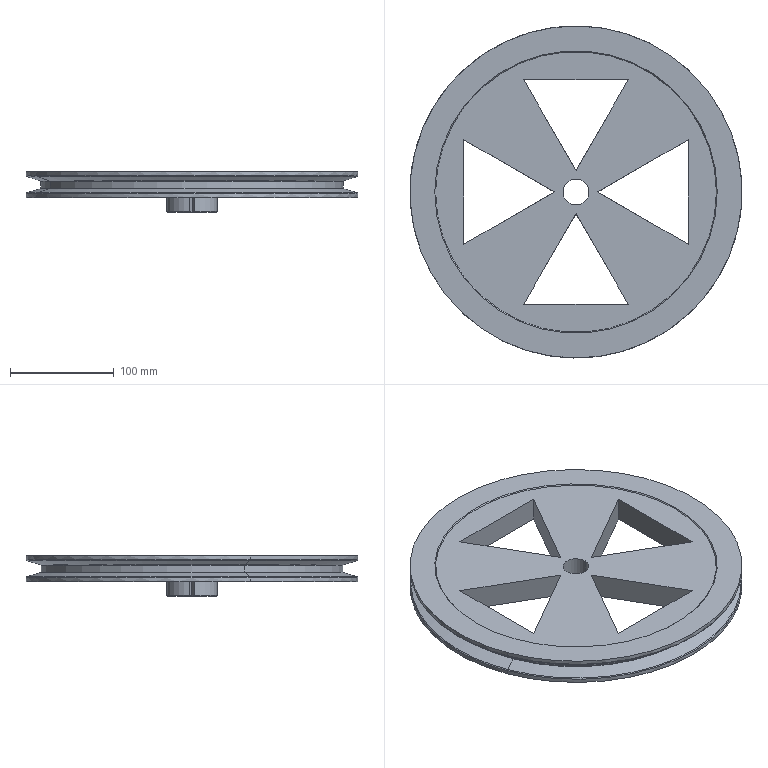Part | SolidWorks | features Fillet 3, ICE 2, Revolution 2, BaseBody 1, HoleWzd 1, RevCut 1 | 1 solid | 51 faces | box 320 x 320 x 39 mm | volume 1356183 mm3 | plane 17 | cylinder 14 | torus 12 | cone 8 | commonest cylinder face diameters 49 x4 320 x4 25 x2 270.571 x2 291.4 x2